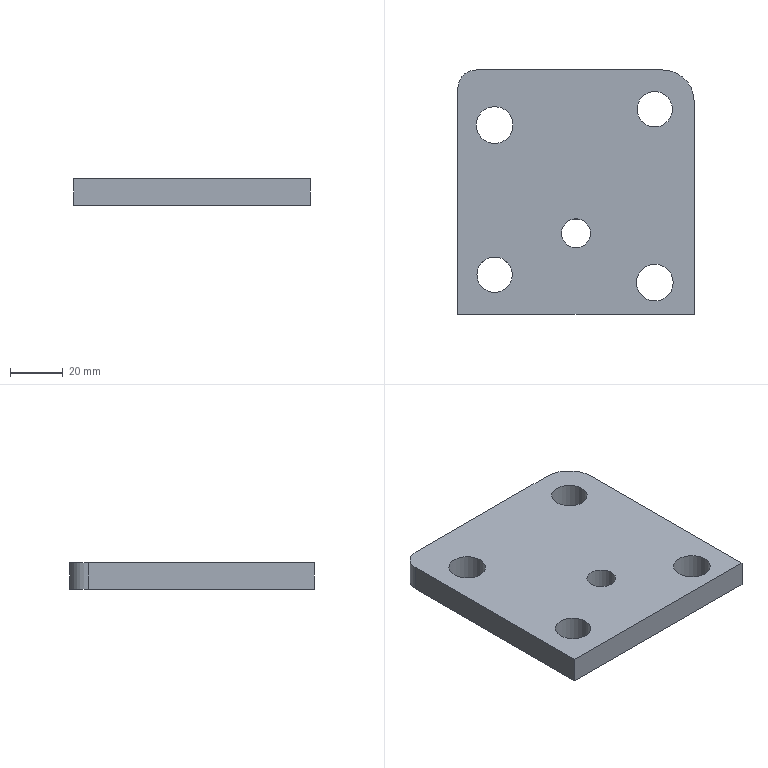Part | STEP file | lll_id2950_x_t | 1 solid | 13 faces | box 90 x 93 x 10 mm | volume 76388 mm3 | cylinder 7 | plane 6 | commonest cylinder face diameters 14 x3 13.509 x2 11.009 x1 24 x1
STEP:
#1=CARTESIAN_POINT('',(928.,-45.25,92.5));
#2=VERTEX_POINT('',#1);
#3=CARTESIAN_POINT('',(921.,-45.25,92.5));
#4=DIRECTION('',(0.,0.,1.));
#5=DIRECTION('',(1.,0.,0.));
#6=AXIS2_PLACEMENT_3D('',#3,#4,#5);
#7=CIRCLE('',#6,7.);
#8=EDGE_CURVE('',#2,#2,#7,.T.);
#9=ORIENTED_EDGE('',*,*,#8,.T.);
#10=EDGE_LOOP('',(#9));
#11=FACE_BOUND('',#10,.T.);
#12=CARTESIAN_POINT('',(927.754,20.75,92.5));
#13=VERTEX_POINT('',#12);
#14=CARTESIAN_POINT('',(921.,20.75,92.5));
#15=DIRECTION('',(0.,0.,-1.));
#16=DIRECTION('',(1.,0.,0.));
#17=AXIS2_PLACEMENT_3D('',#14,#15,#16);
#18=CIRCLE('',#17,6.755);
#19=EDGE_CURVE('',#13,#13,#18,.T.);
#20=ORIENTED_EDGE('',*,*,#19,.F.);
#21=EDGE_LOOP('',(#20));
#22=FACE_BOUND('',#21,.T.);
#23=CARTESIAN_POINT('',(846.,28.75,92.5));
#24=VERTEX_POINT('',#23);
#25=CARTESIAN_POINT('',(846.,-57.25,92.5));
#26=VERTEX_POINT('',#25);
#27=CARTESIAN_POINT('',(846.,-8.25,92.5));
#28=DIRECTION('',(0.,-1.,0.));
#29=VECTOR('',#28,1.);
#30=LINE('',#27,#29);
#31=EDGE_CURVE('',#24,#26,#30,.T.);
#32=ORIENTED_EDGE('',*,*,#31,.F.);
#33=CARTESIAN_POINT('',(853.,35.75,92.5));
#34=VERTEX_POINT('',#33);
#35=CARTESIAN_POINT('',(853.,28.75,92.5));
#36=DIRECTION('',(0.,0.,-1.));
#37=DIRECTION('',(-1.,0.,0.));
#38=AXIS2_PLACEMENT_3D('',#35,#36,#37);
#39=CIRCLE('',#38,7.);
#40=EDGE_CURVE('',#24,#34,#39,.T.);
#41=ORIENTED_EDGE('',*,*,#40,.T.);
#42=CARTESIAN_POINT('',(924.,35.75,92.5));
#43=VERTEX_POINT('',#42);
#44=CARTESIAN_POINT('',(891.,35.75,92.5));
#45=DIRECTION('',(-1.,0.,0.));
#46=VECTOR('',#45,1.);
#47=LINE('',#44,#46);
#48=EDGE_CURVE('',#43,#34,#47,.T.);
#49=ORIENTED_EDGE('',*,*,#48,.F.);
#50=CARTESIAN_POINT('',(936.,23.75,92.5));
#51=VERTEX_POINT('',#50);
#52=CARTESIAN_POINT('',(924.,23.75,92.5));
#53=DIRECTION('',(0.,0.,-1.));
#54=DIRECTION('',(-1.,0.,0.));
#55=AXIS2_PLACEMENT_3D('',#52,#53,#54);
#56=CIRCLE('',#55,12.);
#57=EDGE_CURVE('',#43,#51,#56,.T.);
#58=ORIENTED_EDGE('',*,*,#57,.T.);
#59=CARTESIAN_POINT('',(936.,-57.25,92.5));
#60=VERTEX_POINT('',#59);
#61=CARTESIAN_POINT('',(936.,-8.25,92.5));
#62=DIRECTION('',(0.,1.,0.));
#63=VECTOR('',#62,1.);
#64=LINE('',#61,#63);
#65=EDGE_CURVE('',#60,#51,#64,.T.);
#66=ORIENTED_EDGE('',*,*,#65,.F.);
#67=CARTESIAN_POINT('',(891.,-57.25,92.5));
#68=DIRECTION('',(1.,0.,0.));
#69=VECTOR('',#68,1.);
#70=LINE('',#67,#69);
#71=EDGE_CURVE('',#26,#60,#70,.T.);
#72=ORIENTED_EDGE('',*,*,#71,.F.);
#73=EDGE_LOOP('',(#32,#41,#49,#58,#66,#72));
#74=FACE_BOUND('',#73,.T.);
#75=CARTESIAN_POINT('',(866.754,-42.25,92.5));
#76=VERTEX_POINT('',#75);
#77=CARTESIAN_POINT('',(860.,-42.25,92.5));
#78=DIRECTION('',(0.,0.,-1.));
#79=DIRECTION('',(1.,0.,0.));
#80=AXIS2_PLACEMENT_3D('',#77,#78,#79);
#81=CIRCLE('',#80,6.755);
#82=EDGE_CURVE('',#76,#76,#81,.T.);
#83=ORIENTED_EDGE('',*,*,#82,.F.);
#84=EDGE_LOOP('',(#83));
#85=FACE_BOUND('',#84,.T.);
#86=CARTESIAN_POINT('',(853.,14.75,92.5));
#87=VERTEX_POINT('',#86);
#88=CARTESIAN_POINT('',(860.,14.75,92.5));
#89=DIRECTION('',(0.,0.,1.));
#90=DIRECTION('',(-1.,0.,0.));
#91=AXIS2_PLACEMENT_3D('',#88,#89,#90);
#92=CIRCLE('',#91,7.);
#93=EDGE_CURVE('',#87,#87,#92,.T.);
#94=ORIENTED_EDGE('',*,*,#93,.T.);
#95=EDGE_LOOP('',(#94));
#96=FACE_BOUND('',#95,.T.);
#97=CARTESIAN_POINT('',(885.495,-26.5,92.5));
#98=VERTEX_POINT('',#97);
#99=CARTESIAN_POINT('',(891.,-26.5,92.5));
#100=DIRECTION('',(0.,0.,1.));
#101=DIRECTION('',(-1.,0.,0.));
#102=AXIS2_PLACEMENT_3D('',#99,#100,#101);
#103=CIRCLE('',#102,5.505);
#104=EDGE_CURVE('',#98,#98,#103,.T.);
#105=ORIENTED_EDGE('',*,*,#104,.T.);
#106=EDGE_LOOP('',(#105));
#107=FACE_BOUND('',#106,.T.);
#108=CARTESIAN_POINT('',(891.,-8.25,92.5));
#109=DIRECTION('',(0.,0.,-1.));
#110=DIRECTION('',(1.,0.,0.));
#111=AXIS2_PLACEMENT_3D('',#108,#109,#110);
#112=PLANE('',#111);
#113=ADVANCED_FACE('',(#11,#22,#74,#85,#96,#107),#112,.T.);
#114=CARTESIAN_POINT('',(914.245,20.75,102.5));
#115=VERTEX_POINT('',#114);
#116=CARTESIAN_POINT('',(921.,20.75,102.5));
#117=DIRECTION('',(0.,0.,1.));
#118=DIRECTION('',(-1.,0.,0.));
#119=AXIS2_PLACEMENT_3D('',#116,#117,#118);
#120=CIRCLE('',#119,6.755);
#121=EDGE_CURVE('',#115,#115,#120,.T.);
#122=ORIENTED_EDGE('',*,*,#121,.T.);
#123=EDGE_LOOP('',(#122));
#124=FACE_BOUND('',#123,.T.);
#125=ORIENTED_EDGE('',*,*,#19,.T.);
#126=EDGE_LOOP('',(#125));
#127=FACE_BOUND('',#126,.T.);
#128=CARTESIAN_POINT('',(921.,20.75,57.5));
#129=DIRECTION('',(0.,0.,1.));
#130=DIRECTION('',(1.,0.,0.));
#131=AXIS2_PLACEMENT_3D('',#128,#129,#130);
#132=CYLINDRICAL_SURFACE('',#131,6.755);
#133=ADVANCED_FACE('',(#124,#127),#132,.F.);
#134=CARTESIAN_POINT('',(846.,-57.25,102.5));
#135=VERTEX_POINT('',#134);
#136=CARTESIAN_POINT('',(846.,28.75,102.5));
#137=VERTEX_POINT('',#136);
#138=CARTESIAN_POINT('',(846.,-8.25,102.5));
#139=DIRECTION('',(0.,1.,0.));
#140=VECTOR('',#139,1.);
#141=LINE('',#138,#140);
#142=EDGE_CURVE('',#135,#137,#141,.T.);
#143=ORIENTED_EDGE('',*,*,#142,.T.);
#144=CARTESIAN_POINT('',(846.,28.75,92.5));
#145=DIRECTION('',(0.,0.,-1.));
#146=VECTOR('',#145,1.);
#147=LINE('',#144,#146);
#148=EDGE_CURVE('',#137,#24,#147,.T.);
#149=ORIENTED_EDGE('',*,*,#148,.T.);
#150=ORIENTED_EDGE('',*,*,#31,.T.);
#151=CARTESIAN_POINT('',(846.,-57.25,92.5));
#152=DIRECTION('',(0.,0.,1.));
#153=VECTOR('',#152,1.);
#154=LINE('',#151,#153);
#155=EDGE_CURVE('',#26,#135,#154,.T.);
#156=ORIENTED_EDGE('',*,*,#155,.T.);
#157=EDGE_LOOP('',(#143,#149,#150,#156));
#158=FACE_OUTER_BOUND('',#157,.T.);
#159=CARTESIAN_POINT('',(846.,-8.25,92.5));
#160=DIRECTION('',(-1.,0.,0.));
#161=DIRECTION('',(0.,0.,-1.));
#162=AXIS2_PLACEMENT_3D('',#159,#160,#161);
#163=PLANE('',#162);
#164=ADVANCED_FACE('',(#158),#163,.T.);
#165=CARTESIAN_POINT('',(936.,-57.25,102.5));
#166=VERTEX_POINT('',#165);
#167=CARTESIAN_POINT('',(891.,-57.25,102.5));
#168=DIRECTION('',(1.,0.,0.));
#169=VECTOR('',#168,1.);
#170=LINE('',#167,#169);
#171=EDGE_CURVE('',#135,#166,#170,.T.);
#172=ORIENTED_EDGE('',*,*,#171,.F.);
#173=ORIENTED_EDGE('',*,*,#155,.F.);
#174=ORIENTED_EDGE('',*,*,#71,.T.);
#175=CARTESIAN_POINT('',(936.,-57.25,92.5));
#176=DIRECTION('',(0.,0.,1.));
#177=VECTOR('',#176,1.);
#178=LINE('',#175,#177);
#179=EDGE_CURVE('',#60,#166,#178,.T.);
#180=ORIENTED_EDGE('',*,*,#179,.T.);
#181=EDGE_LOOP('',(#172,#173,#174,#180));
#182=FACE_OUTER_BOUND('',#181,.T.);
#183=CARTESIAN_POINT('',(891.,-57.25,92.5));
#184=DIRECTION('',(0.,-1.,0.));
#185=DIRECTION('',(0.,0.,1.));
#186=AXIS2_PLACEMENT_3D('',#183,#184,#185);
#187=PLANE('',#186);
#188=ADVANCED_FACE('',(#182),#187,.T.);
#189=ORIENTED_EDGE('',*,*,#65,.T.);
#190=CARTESIAN_POINT('',(936.,23.75,102.5));
#191=VERTEX_POINT('',#190);
#192=CARTESIAN_POINT('',(936.,23.75,92.5));
#193=DIRECTION('',(0.,0.,1.));
#194=VECTOR('',#193,1.);
#195=LINE('',#192,#194);
#196=EDGE_CURVE('',#51,#191,#195,.T.);
#197=ORIENTED_EDGE('',*,*,#196,.T.);
#198=CARTESIAN_POINT('',(936.,-8.25,102.5));
#199=DIRECTION('',(0.,-1.,0.));
#200=VECTOR('',#199,1.);
#201=LINE('',#198,#200);
#202=EDGE_CURVE('',#191,#166,#201,.T.);
#203=ORIENTED_EDGE('',*,*,#202,.T.);
#204=ORIENTED_EDGE('',*,*,#179,.F.);
#205=EDGE_LOOP('',(#189,#197,#203,#204));
#206=FACE_OUTER_BOUND('',#205,.T.);
#207=CARTESIAN_POINT('',(936.,-8.25,92.5));
#208=DIRECTION('',(1.,0.,0.));
#209=DIRECTION('',(0.,0.,1.));
#210=AXIS2_PLACEMENT_3D('',#207,#208,#209);
#211=PLANE('',#210);
#212=ADVANCED_FACE('',(#206),#211,.T.);
#213=ORIENTED_EDGE('',*,*,#48,.T.);
#214=CARTESIAN_POINT('',(853.,35.75,102.5));
#215=VERTEX_POINT('',#214);
#216=CARTESIAN_POINT('',(853.,35.75,92.5));
#217=DIRECTION('',(0.,0.,1.));
#218=VECTOR('',#217,1.);
#219=LINE('',#216,#218);
#220=EDGE_CURVE('',#34,#215,#219,.T.);
#221=ORIENTED_EDGE('',*,*,#220,.T.);
#222=CARTESIAN_POINT('',(924.,35.75,102.5));
#223=VERTEX_POINT('',#222);
#224=CARTESIAN_POINT('',(891.,35.75,102.5));
#225=DIRECTION('',(1.,0.,0.));
#226=VECTOR('',#225,1.);
#227=LINE('',#224,#226);
#228=EDGE_CURVE('',#215,#223,#227,.T.);
#229=ORIENTED_EDGE('',*,*,#228,.T.);
#230=CARTESIAN_POINT('',(924.,35.75,92.5));
#231=DIRECTION('',(0.,0.,-1.));
#232=VECTOR('',#231,1.);
#233=LINE('',#230,#232);
#234=EDGE_CURVE('',#223,#43,#233,.T.);
#235=ORIENTED_EDGE('',*,*,#234,.T.);
#236=EDGE_LOOP('',(#213,#221,#229,#235));
#237=FACE_OUTER_BOUND('',#236,.T.);
#238=CARTESIAN_POINT('',(891.,35.75,92.5));
#239=DIRECTION('',(0.,1.,0.));
#240=DIRECTION('',(0.,0.,-1.));
#241=AXIS2_PLACEMENT_3D('',#238,#239,#240);
#242=PLANE('',#241);
#243=ADVANCED_FACE('',(#237),#242,.T.);
#244=CARTESIAN_POINT('',(853.245,-42.25,102.5));
#245=VERTEX_POINT('',#244);
#246=CARTESIAN_POINT('',(860.,-42.25,102.5));
#247=DIRECTION('',(0.,0.,1.));
#248=DIRECTION('',(-1.,0.,0.));
#249=AXIS2_PLACEMENT_3D('',#246,#247,#248);
#250=CIRCLE('',#249,6.755);
#251=EDGE_CURVE('',#245,#245,#250,.T.);
#252=ORIENTED_EDGE('',*,*,#251,.T.);
#253=EDGE_LOOP('',(#252));
#254=FACE_BOUND('',#253,.T.);
#255=ORIENTED_EDGE('',*,*,#82,.T.);
#256=EDGE_LOOP('',(#255));
#257=FACE_BOUND('',#256,.T.);
#258=CARTESIAN_POINT('',(860.,-42.25,57.5));
#259=DIRECTION('',(0.,0.,1.));
#260=DIRECTION('',(-1.,0.,0.));
#261=AXIS2_PLACEMENT_3D('',#258,#259,#260);
#262=CYLINDRICAL_SURFACE('',#261,6.755);
#263=ADVANCED_FACE('',(#254,#257),#262,.F.);
#264=CARTESIAN_POINT('',(853.,14.75,102.5));
#265=VERTEX_POINT('',#264);
#266=CARTESIAN_POINT('',(860.,14.75,102.5));
#267=DIRECTION('',(0.,0.,1.));
#268=DIRECTION('',(-1.,0.,0.));
#269=AXIS2_PLACEMENT_3D('',#266,#267,#268);
#270=CIRCLE('',#269,7.);
#271=EDGE_CURVE('',#265,#265,#270,.T.);
#272=ORIENTED_EDGE('',*,*,#271,.T.);
#273=EDGE_LOOP('',(#272));
#274=FACE_BOUND('',#273,.T.);
#275=ORIENTED_EDGE('',*,*,#93,.F.);
#276=EDGE_LOOP('',(#275));
#277=FACE_BOUND('',#276,.T.);
#278=CARTESIAN_POINT('',(860.,14.75,92.5));
#279=DIRECTION('',(0.,0.,1.));
#280=DIRECTION('',(-1.,0.,0.));
#281=AXIS2_PLACEMENT_3D('',#278,#279,#280);
#282=CYLINDRICAL_SURFACE('',#281,7.);
#283=ADVANCED_FACE('',(#274,#277),#282,.F.);
#284=CARTESIAN_POINT('',(914.,-45.25,102.5));
#285=VERTEX_POINT('',#284);
#286=CARTESIAN_POINT('',(921.,-45.25,102.5));
#287=DIRECTION('',(0.,0.,1.));
#288=DIRECTION('',(-1.,0.,0.));
#289=AXIS2_PLACEMENT_3D('',#286,#287,#288);
#290=CIRCLE('',#289,7.);
#291=EDGE_CURVE('',#285,#285,#290,.T.);
#292=ORIENTED_EDGE('',*,*,#291,.T.);
#293=EDGE_LOOP('',(#292));
#294=FACE_BOUND('',#293,.T.);
#295=ORIENTED_EDGE('',*,*,#8,.F.);
#296=EDGE_LOOP('',(#295));
#297=FACE_BOUND('',#296,.T.);
#298=CARTESIAN_POINT('',(921.,-45.25,92.5));
#299=DIRECTION('',(0.,0.,1.));
#300=DIRECTION('',(1.,0.,0.));
#301=AXIS2_PLACEMENT_3D('',#298,#299,#300);
#302=CYLINDRICAL_SURFACE('',#301,7.);
#303=ADVANCED_FACE('',(#294,#297),#302,.F.);
#304=CARTESIAN_POINT('',(885.495,-26.5,102.5));
#305=VERTEX_POINT('',#304);
#306=CARTESIAN_POINT('',(891.,-26.5,102.5));
#307=DIRECTION('',(0.,0.,-1.));
#308=DIRECTION('',(-1.,0.,0.));
#309=AXIS2_PLACEMENT_3D('',#306,#307,#308);
#310=CIRCLE('',#309,5.505);
#311=EDGE_CURVE('',#305,#305,#310,.T.);
#312=ORIENTED_EDGE('',*,*,#311,.T.);
#313=EDGE_LOOP('',(#312));
#314=FACE_BOUND('',#313,.T.);
#315=ORIENTED_EDGE('',*,*,#228,.F.);
#316=CARTESIAN_POINT('',(853.,28.75,102.5));
#317=DIRECTION('',(0.,0.,1.));
#318=DIRECTION('',(-1.,0.,0.));
#319=AXIS2_PLACEMENT_3D('',#316,#317,#318);
#320=CIRCLE('',#319,7.);
#321=EDGE_CURVE('',#215,#137,#320,.T.);
#322=ORIENTED_EDGE('',*,*,#321,.T.);
#323=ORIENTED_EDGE('',*,*,#142,.F.);
#324=ORIENTED_EDGE('',*,*,#171,.T.);
#325=ORIENTED_EDGE('',*,*,#202,.F.);
#326=CARTESIAN_POINT('',(924.,23.75,102.5));
#327=DIRECTION('',(0.,0.,1.));
#328=DIRECTION('',(-1.,0.,0.));
#329=AXIS2_PLACEMENT_3D('',#326,#327,#328);
#330=CIRCLE('',#329,12.);
#331=EDGE_CURVE('',#191,#223,#330,.T.);
#332=ORIENTED_EDGE('',*,*,#331,.T.);
#333=EDGE_LOOP('',(#315,#322,#323,#324,#325,#332));
#334=FACE_BOUND('',#333,.T.);
#335=ORIENTED_EDGE('',*,*,#271,.F.);
#336=EDGE_LOOP('',(#335));
#337=FACE_BOUND('',#336,.T.);
#338=ORIENTED_EDGE('',*,*,#291,.F.);
#339=EDGE_LOOP('',(#338));
#340=FACE_BOUND('',#339,.T.);
#341=ORIENTED_EDGE('',*,*,#121,.F.);
#342=EDGE_LOOP('',(#341));
#343=FACE_BOUND('',#342,.T.);
#344=ORIENTED_EDGE('',*,*,#251,.F.);
#345=EDGE_LOOP('',(#344));
#346=FACE_BOUND('',#345,.T.);
#347=CARTESIAN_POINT('',(741.5,-0.002299,102.5));
#348=DIRECTION('',(0.,0.,-1.));
#349=DIRECTION('',(-1.,0.,0.));
#350=AXIS2_PLACEMENT_3D('',#347,#348,#349);
#351=PLANE('',#350);
#352=ADVANCED_FACE('',(#314,#334,#337,#340,#343,#346),#351,.F.);
#353=ORIENTED_EDGE('',*,*,#104,.F.);
#354=EDGE_LOOP('',(#353));
#355=FACE_BOUND('',#354,.T.);
#356=ORIENTED_EDGE('',*,*,#311,.F.);
#357=EDGE_LOOP('',(#356));
#358=FACE_BOUND('',#357,.T.);
#359=CARTESIAN_POINT('',(891.,-26.5,92.5));
#360=DIRECTION('',(0.,0.,1.));
#361=DIRECTION('',(1.,0.,0.));
#362=AXIS2_PLACEMENT_3D('',#359,#360,#361);
#363=CYLINDRICAL_SURFACE('',#362,5.505);
#364=ADVANCED_FACE('',(#355,#358),#363,.F.);
#365=ORIENTED_EDGE('',*,*,#57,.F.);
#366=ORIENTED_EDGE('',*,*,#234,.F.);
#367=ORIENTED_EDGE('',*,*,#331,.F.);
#368=ORIENTED_EDGE('',*,*,#196,.F.);
#369=EDGE_LOOP('',(#365,#366,#367,#368));
#370=FACE_OUTER_BOUND('',#369,.T.);
#371=CARTESIAN_POINT('',(924.,23.75,92.5));
#372=DIRECTION('',(0.,0.,1.));
#373=DIRECTION('',(1.,0.,0.));
#374=AXIS2_PLACEMENT_3D('',#371,#372,#373);
#375=CYLINDRICAL_SURFACE('',#374,12.);
#376=ADVANCED_FACE('',(#370),#375,.T.);
#377=ORIENTED_EDGE('',*,*,#40,.F.);
#378=ORIENTED_EDGE('',*,*,#148,.F.);
#379=ORIENTED_EDGE('',*,*,#321,.F.);
#380=ORIENTED_EDGE('',*,*,#220,.F.);
#381=EDGE_LOOP('',(#377,#378,#379,#380));
#382=FACE_OUTER_BOUND('',#381,.T.);
#383=CARTESIAN_POINT('',(853.,28.75,92.5));
#384=DIRECTION('',(0.,0.,1.));
#385=DIRECTION('',(1.,0.,0.));
#386=AXIS2_PLACEMENT_3D('',#383,#384,#385);
#387=CYLINDRICAL_SURFACE('',#386,7.);
#388=ADVANCED_FACE('',(#382),#387,.T.);
#389=CLOSED_SHELL('',(#113,#133,#164,#188,#212,#243,#263,#283,#303,#352,#364,#376,#388));
#390=MANIFOLD_SOLID_BREP('',#389);
#391=(LENGTH_UNIT()NAMED_UNIT(*)SI_UNIT(.MILLI.,.METRE.));
#392=UNCERTAINTY_MEASURE_WITH_UNIT(LENGTH_MEASURE(0.00002),#391,'','');
#393=(NAMED_UNIT(*)PLANE_ANGLE_UNIT()SI_UNIT($,.RADIAN.));
#394=PLANE_ANGLE_MEASURE_WITH_UNIT(PLANE_ANGLE_MEASURE(0.01745),#393);
#395=DIMENSIONAL_EXPONENTS(0.,0.,0.,0.,0.,0.,0.);
#396=(CONVERSION_BASED_UNIT('DEGREE',#394)NAMED_UNIT(#395)PLANE_ANGLE_UNIT());
#397=(NAMED_UNIT(*)SI_UNIT($,.STERADIAN.)SOLID_ANGLE_UNIT());
#398=(GEOMETRIC_REPRESENTATION_CONTEXT(3)GLOBAL_UNCERTAINTY_ASSIGNED_CONTEXT((#392))GLOBAL_UNIT_ASSIGNED_CONTEXT((#391,#396,#397))REPRESENTATION_CONTEXT('',''));
#399=ADVANCED_BREP_SHAPE_REPRESENTATION('',(#390),#398);